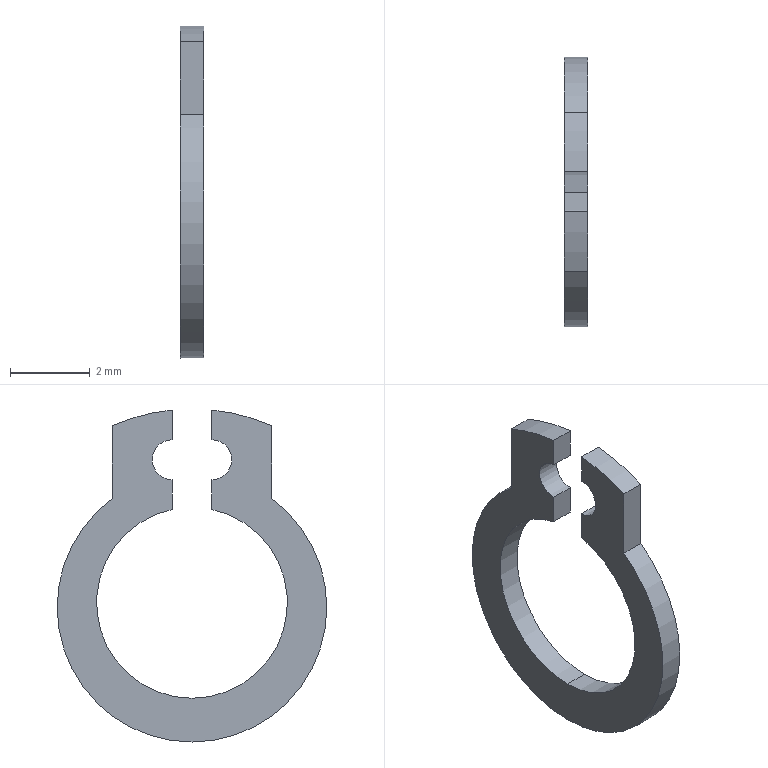Part | SolidWorks | features BaseBody 1 | 1 solid | 16 faces | box 0.6 x 6.78 x 8.347 mm | volume 12.837 mm3 | cylinder 8 | plane 8 | commonest cylinder face diameters 1 x2 4.8 x2 6.78 x2 9.965 x2
STEP:
#1=CARTESIAN_POINT('',(487.737,38.215,67.713));
#2=VERTEX_POINT('',#1);
#3=CARTESIAN_POINT('',(487.737,37.715,62.966));
#4=VERTEX_POINT('',#3);
#5=CARTESIAN_POINT('',(487.737,37.715,65.366));
#6=DIRECTION('',(-1.,0.,-0.000000013));
#7=DIRECTION('',(0.000000013,0.,-1.));
#8=AXIS2_PLACEMENT_3D('',#5,#6,#7);
#9=CIRCLE('',#8,2.4);
#10=EDGE_CURVE('',#2,#4,#9,.T.);
#11=ORIENTED_EDGE('',*,*,#10,.T.);
#12=CARTESIAN_POINT('',(488.337,37.715,62.966));
#13=VERTEX_POINT('',#12);
#14=CARTESIAN_POINT('',(487.737,37.715,62.966));
#15=DIRECTION('',(1.,0.,0.000000013));
#16=VECTOR('',#15,1000.);
#17=LINE('',#14,#16);
#18=EDGE_CURVE('',#4,#13,#17,.T.);
#19=ORIENTED_EDGE('',*,*,#18,.T.);
#20=CARTESIAN_POINT('',(488.337,38.215,67.713));
#21=VERTEX_POINT('',#20);
#22=CARTESIAN_POINT('',(488.337,37.715,65.366));
#23=DIRECTION('',(1.,0.,0.000000013));
#24=DIRECTION('',(0.000000013,0.,-1.));
#25=AXIS2_PLACEMENT_3D('',#22,#23,#24);
#26=CIRCLE('',#25,2.4);
#27=EDGE_CURVE('',#13,#21,#26,.T.);
#28=ORIENTED_EDGE('',*,*,#27,.T.);
#29=CARTESIAN_POINT('',(488.037,38.215,67.713));
#30=DIRECTION('',(-1.,0.,-0.000000013));
#31=VECTOR('',#30,1000.);
#32=LINE('',#29,#31);
#33=EDGE_CURVE('',#21,#2,#32,.T.);
#34=ORIENTED_EDGE('',*,*,#33,.T.);
#35=EDGE_LOOP('',(#11,#19,#28,#34));
#36=FACE_OUTER_BOUND('',#35,.T.);
#37=CARTESIAN_POINT('',(487.737,37.715,65.366));
#38=DIRECTION('',(1.,0.,0.000000013));
#39=DIRECTION('',(0.000000013,0.,-1.));
#40=AXIS2_PLACEMENT_3D('',#37,#38,#39);
#41=CYLINDRICAL_SURFACE('',#40,2.4);
#42=ADVANCED_FACE('',(#36),#41,.F.);
#43=CARTESIAN_POINT('',(487.737,35.715,67.993));
#44=VERTEX_POINT('',#43);
#45=CARTESIAN_POINT('',(487.737,37.715,61.866));
#46=VERTEX_POINT('',#45);
#47=CARTESIAN_POINT('',(487.737,37.715,65.256));
#48=DIRECTION('',(1.,0.,0.000000013));
#49=DIRECTION('',(0.000000013,0.,-1.));
#50=AXIS2_PLACEMENT_3D('',#47,#48,#49);
#51=CIRCLE('',#50,3.39);
#52=EDGE_CURVE('',#44,#46,#51,.T.);
#53=ORIENTED_EDGE('',*,*,#52,.T.);
#54=CARTESIAN_POINT('',(488.337,37.715,61.866));
#55=VERTEX_POINT('',#54);
#56=CARTESIAN_POINT('',(487.737,37.715,61.866));
#57=DIRECTION('',(1.,0.,0.000000013));
#58=VECTOR('',#57,1000.);
#59=LINE('',#56,#58);
#60=EDGE_CURVE('',#46,#55,#59,.T.);
#61=ORIENTED_EDGE('',*,*,#60,.T.);
#62=CARTESIAN_POINT('',(488.337,35.715,67.993));
#63=VERTEX_POINT('',#62);
#64=CARTESIAN_POINT('',(488.337,37.715,65.256));
#65=DIRECTION('',(1.,0.,0.000000013));
#66=DIRECTION('',(0.000000013,0.,-1.));
#67=AXIS2_PLACEMENT_3D('',#64,#65,#66);
#68=CIRCLE('',#67,3.39);
#69=EDGE_CURVE('',#63,#55,#68,.T.);
#70=ORIENTED_EDGE('',*,*,#69,.F.);
#71=CARTESIAN_POINT('',(488.037,35.715,67.993));
#72=DIRECTION('',(1.,0.,0.000000013));
#73=VECTOR('',#72,1000.);
#74=LINE('',#71,#73);
#75=EDGE_CURVE('',#44,#63,#74,.T.);
#76=ORIENTED_EDGE('',*,*,#75,.F.);
#77=EDGE_LOOP('',(#53,#61,#70,#76));
#78=FACE_OUTER_BOUND('',#77,.T.);
#79=CARTESIAN_POINT('',(487.737,37.715,65.256));
#80=DIRECTION('',(1.,0.,0.000000013));
#81=DIRECTION('',(0.000000013,0.,-1.));
#82=AXIS2_PLACEMENT_3D('',#79,#80,#81);
#83=CYLINDRICAL_SURFACE('',#82,3.39);
#84=ADVANCED_FACE('',(#78),#83,.T.);
#85=CARTESIAN_POINT('',(487.737,37.215,68.463));
#86=VERTEX_POINT('',#85);
#87=CARTESIAN_POINT('',(487.737,37.215,69.463));
#88=VERTEX_POINT('',#87);
#89=CARTESIAN_POINT('',(487.737,37.215,68.963));
#90=DIRECTION('',(-1.,0.,-0.000000013));
#91=DIRECTION('',(0.000000013,0.,-1.));
#92=AXIS2_PLACEMENT_3D('',#89,#90,#91);
#93=CIRCLE('',#92,0.5);
#94=EDGE_CURVE('',#86,#88,#93,.T.);
#95=ORIENTED_EDGE('',*,*,#94,.F.);
#96=CARTESIAN_POINT('',(487.737,37.215,67.713));
#97=VERTEX_POINT('',#96);
#98=CARTESIAN_POINT('',(487.737,37.215,66.04));
#99=DIRECTION('',(-0.000000013,0.,1.));
#100=VECTOR('',#99,1000.);
#101=LINE('',#98,#100);
#102=EDGE_CURVE('',#97,#86,#101,.T.);
#103=ORIENTED_EDGE('',*,*,#102,.F.);
#104=CARTESIAN_POINT('',(487.737,37.715,65.366));
#105=DIRECTION('',(-1.,0.,-0.000000013));
#106=DIRECTION('',(0.000000013,0.,-1.));
#107=AXIS2_PLACEMENT_3D('',#104,#105,#106);
#108=CIRCLE('',#107,2.4);
#109=EDGE_CURVE('',#4,#97,#108,.T.);
#110=ORIENTED_EDGE('',*,*,#109,.F.);
#111=ORIENTED_EDGE('',*,*,#10,.F.);
#112=CARTESIAN_POINT('',(487.737,38.215,68.463));
#113=VERTEX_POINT('',#112);
#114=CARTESIAN_POINT('',(487.737,38.215,66.04));
#115=DIRECTION('',(0.000000013,0.,-1.));
#116=VECTOR('',#115,1000.);
#117=LINE('',#114,#116);
#118=EDGE_CURVE('',#113,#2,#117,.T.);
#119=ORIENTED_EDGE('',*,*,#118,.F.);
#120=CARTESIAN_POINT('',(487.737,38.215,69.463));
#121=VERTEX_POINT('',#120);
#122=CARTESIAN_POINT('',(487.737,38.215,68.963));
#123=DIRECTION('',(-1.,0.,-0.000000013));
#124=DIRECTION('',(0.000000013,0.,-1.));
#125=AXIS2_PLACEMENT_3D('',#122,#123,#124);
#126=CIRCLE('',#125,0.5);
#127=EDGE_CURVE('',#121,#113,#126,.T.);
#128=ORIENTED_EDGE('',*,*,#127,.F.);
#129=CARTESIAN_POINT('',(487.737,38.215,70.213));
#130=VERTEX_POINT('',#129);
#131=CARTESIAN_POINT('',(487.737,38.215,66.04));
#132=DIRECTION('',(0.000000013,0.,-1.));
#133=VECTOR('',#132,1000.);
#134=LINE('',#131,#133);
#135=EDGE_CURVE('',#130,#121,#134,.T.);
#136=ORIENTED_EDGE('',*,*,#135,.F.);
#137=CARTESIAN_POINT('',(487.737,39.715,69.819));
#138=VERTEX_POINT('',#137);
#139=CARTESIAN_POINT('',(487.737,37.715,65.256));
#140=DIRECTION('',(1.,0.,0.000000013));
#141=DIRECTION('',(0.000000013,0.,-1.));
#142=AXIS2_PLACEMENT_3D('',#139,#140,#141);
#143=CIRCLE('',#142,4.982);
#144=EDGE_CURVE('',#138,#130,#143,.T.);
#145=ORIENTED_EDGE('',*,*,#144,.F.);
#146=CARTESIAN_POINT('',(487.737,39.715,67.993));
#147=VERTEX_POINT('',#146);
#148=CARTESIAN_POINT('',(487.737,39.715,66.04));
#149=DIRECTION('',(-0.000000013,0.,1.));
#150=VECTOR('',#149,1000.);
#151=LINE('',#148,#150);
#152=EDGE_CURVE('',#147,#138,#151,.T.);
#153=ORIENTED_EDGE('',*,*,#152,.F.);
#154=CARTESIAN_POINT('',(487.737,37.715,65.256));
#155=DIRECTION('',(1.,0.,0.000000013));
#156=DIRECTION('',(0.000000013,0.,-1.));
#157=AXIS2_PLACEMENT_3D('',#154,#155,#156);
#158=CIRCLE('',#157,3.39);
#159=EDGE_CURVE('',#46,#147,#158,.T.);
#160=ORIENTED_EDGE('',*,*,#159,.F.);
#161=ORIENTED_EDGE('',*,*,#52,.F.);
#162=CARTESIAN_POINT('',(487.737,35.715,69.819));
#163=VERTEX_POINT('',#162);
#164=CARTESIAN_POINT('',(487.737,35.715,66.04));
#165=DIRECTION('',(0.000000013,0.,-1.));
#166=VECTOR('',#165,1000.);
#167=LINE('',#164,#166);
#168=EDGE_CURVE('',#163,#44,#167,.T.);
#169=ORIENTED_EDGE('',*,*,#168,.F.);
#170=CARTESIAN_POINT('',(487.737,37.215,70.213));
#171=VERTEX_POINT('',#170);
#172=CARTESIAN_POINT('',(487.737,37.715,65.256));
#173=DIRECTION('',(1.,0.,0.000000013));
#174=DIRECTION('',(0.000000013,0.,-1.));
#175=AXIS2_PLACEMENT_3D('',#172,#173,#174);
#176=CIRCLE('',#175,4.982);
#177=EDGE_CURVE('',#171,#163,#176,.T.);
#178=ORIENTED_EDGE('',*,*,#177,.F.);
#179=CARTESIAN_POINT('',(487.737,37.215,66.04));
#180=DIRECTION('',(-0.000000013,0.,1.));
#181=VECTOR('',#180,1000.);
#182=LINE('',#179,#181);
#183=EDGE_CURVE('',#88,#171,#182,.T.);
#184=ORIENTED_EDGE('',*,*,#183,.F.);
#185=EDGE_LOOP('',(#95,#103,#110,#111,#119,#128,#136,#145,#153,#160,#161,#169,#178,#184));
#186=FACE_OUTER_BOUND('',#185,.T.);
#187=CARTESIAN_POINT('',(487.737,41.317,70.38));
#188=DIRECTION('',(1.,0.,0.000000013));
#189=DIRECTION('',(0.,-1.,0.));
#190=AXIS2_PLACEMENT_3D('',#187,#188,#189);
#191=PLANE('',#190);
#192=ADVANCED_FACE('',(#186),#191,.F.);
#193=CARTESIAN_POINT('',(488.337,37.215,69.463));
#194=VERTEX_POINT('',#193);
#195=CARTESIAN_POINT('',(488.037,37.215,69.463));
#196=DIRECTION('',(1.,0.,0.000000013));
#197=VECTOR('',#196,1000.);
#198=LINE('',#195,#197);
#199=EDGE_CURVE('',#88,#194,#198,.T.);
#200=ORIENTED_EDGE('',*,*,#199,.T.);
#201=CARTESIAN_POINT('',(488.337,37.215,68.463));
#202=VERTEX_POINT('',#201);
#203=CARTESIAN_POINT('',(488.337,37.215,68.963));
#204=DIRECTION('',(-1.,0.,-0.000000013));
#205=DIRECTION('',(0.000000013,0.,-1.));
#206=AXIS2_PLACEMENT_3D('',#203,#204,#205);
#207=CIRCLE('',#206,0.5);
#208=EDGE_CURVE('',#202,#194,#207,.T.);
#209=ORIENTED_EDGE('',*,*,#208,.F.);
#210=CARTESIAN_POINT('',(488.037,37.215,68.463));
#211=DIRECTION('',(-1.,0.,-0.000000013));
#212=VECTOR('',#211,1000.);
#213=LINE('',#210,#212);
#214=EDGE_CURVE('',#202,#86,#213,.T.);
#215=ORIENTED_EDGE('',*,*,#214,.T.);
#216=ORIENTED_EDGE('',*,*,#94,.T.);
#217=EDGE_LOOP('',(#200,#209,#215,#216));
#218=FACE_OUTER_BOUND('',#217,.T.);
#219=CARTESIAN_POINT('',(487.737,37.215,68.963));
#220=DIRECTION('',(1.,0.,0.000000013));
#221=DIRECTION('',(0.000000013,0.,-1.));
#222=AXIS2_PLACEMENT_3D('',#219,#220,#221);
#223=CYLINDRICAL_SURFACE('',#222,0.5);
#224=ADVANCED_FACE('',(#218),#223,.F.);
#225=CARTESIAN_POINT('',(488.337,37.215,67.713));
#226=VERTEX_POINT('',#225);
#227=CARTESIAN_POINT('',(488.037,37.215,67.713));
#228=DIRECTION('',(-1.,0.,-0.000000013));
#229=VECTOR('',#228,1000.);
#230=LINE('',#227,#229);
#231=EDGE_CURVE('',#226,#97,#230,.T.);
#232=ORIENTED_EDGE('',*,*,#231,.T.);
#233=ORIENTED_EDGE('',*,*,#102,.T.);
#234=ORIENTED_EDGE('',*,*,#214,.F.);
#235=CARTESIAN_POINT('',(488.337,37.215,66.04));
#236=DIRECTION('',(-0.000000013,0.,1.));
#237=VECTOR('',#236,1000.);
#238=LINE('',#235,#237);
#239=EDGE_CURVE('',#226,#202,#238,.T.);
#240=ORIENTED_EDGE('',*,*,#239,.F.);
#241=EDGE_LOOP('',(#232,#233,#234,#240));
#242=FACE_OUTER_BOUND('',#241,.T.);
#243=CARTESIAN_POINT('',(487.724,37.215,67.663));
#244=DIRECTION('',(0.,1.,0.));
#245=DIRECTION('',(-0.000000013,0.,1.));
#246=AXIS2_PLACEMENT_3D('',#243,#244,#245);
#247=PLANE('',#246);
#248=ADVANCED_FACE('',(#242),#247,.T.);
#249=ORIENTED_EDGE('',*,*,#18,.F.);
#250=ORIENTED_EDGE('',*,*,#109,.T.);
#251=ORIENTED_EDGE('',*,*,#231,.F.);
#252=CARTESIAN_POINT('',(488.337,37.715,65.366));
#253=DIRECTION('',(1.,0.,0.000000013));
#254=DIRECTION('',(0.000000013,0.,-1.));
#255=AXIS2_PLACEMENT_3D('',#252,#253,#254);
#256=CIRCLE('',#255,2.4);
#257=EDGE_CURVE('',#226,#13,#256,.T.);
#258=ORIENTED_EDGE('',*,*,#257,.T.);
#259=EDGE_LOOP('',(#249,#250,#251,#258));
#260=FACE_OUTER_BOUND('',#259,.T.);
#261=CARTESIAN_POINT('',(487.737,37.715,65.366));
#262=DIRECTION('',(1.,0.,0.000000013));
#263=DIRECTION('',(0.000000013,0.,-1.));
#264=AXIS2_PLACEMENT_3D('',#261,#262,#263);
#265=CYLINDRICAL_SURFACE('',#264,2.4);
#266=ADVANCED_FACE('',(#260),#265,.F.);
#267=ORIENTED_EDGE('',*,*,#33,.F.);
#268=CARTESIAN_POINT('',(488.337,38.215,68.463));
#269=VERTEX_POINT('',#268);
#270=CARTESIAN_POINT('',(488.337,38.215,68.963));
#271=DIRECTION('',(-0.000000013,0.,1.));
#272=VECTOR('',#271,1000.);
#273=LINE('',#270,#272);
#274=EDGE_CURVE('',#21,#269,#273,.T.);
#275=ORIENTED_EDGE('',*,*,#274,.T.);
#276=CARTESIAN_POINT('',(488.037,38.215,68.463));
#277=DIRECTION('',(-1.,0.,-0.000000013));
#278=VECTOR('',#277,1000.);
#279=LINE('',#276,#278);
#280=EDGE_CURVE('',#269,#113,#279,.T.);
#281=ORIENTED_EDGE('',*,*,#280,.T.);
#282=ORIENTED_EDGE('',*,*,#118,.T.);
#283=EDGE_LOOP('',(#267,#275,#281,#282));
#284=FACE_OUTER_BOUND('',#283,.T.);
#285=CARTESIAN_POINT('',(487.724,38.215,70.263));
#286=DIRECTION('',(0.,-1.,0.));
#287=DIRECTION('',(0.000000013,0.,-1.));
#288=AXIS2_PLACEMENT_3D('',#285,#286,#287);
#289=PLANE('',#288);
#290=ADVANCED_FACE('',(#284),#289,.T.);
#291=ORIENTED_EDGE('',*,*,#280,.F.);
#292=CARTESIAN_POINT('',(488.337,38.215,69.463));
#293=VERTEX_POINT('',#292);
#294=CARTESIAN_POINT('',(488.337,38.215,68.963));
#295=DIRECTION('',(1.,0.,0.000000013));
#296=DIRECTION('',(0.000000013,0.,-1.));
#297=AXIS2_PLACEMENT_3D('',#294,#295,#296);
#298=CIRCLE('',#297,0.5);
#299=EDGE_CURVE('',#269,#293,#298,.T.);
#300=ORIENTED_EDGE('',*,*,#299,.T.);
#301=CARTESIAN_POINT('',(488.037,38.215,69.463));
#302=DIRECTION('',(-1.,0.,-0.000000013));
#303=VECTOR('',#302,1000.);
#304=LINE('',#301,#303);
#305=EDGE_CURVE('',#293,#121,#304,.T.);
#306=ORIENTED_EDGE('',*,*,#305,.T.);
#307=ORIENTED_EDGE('',*,*,#127,.T.);
#308=EDGE_LOOP('',(#291,#300,#306,#307));
#309=FACE_OUTER_BOUND('',#308,.T.);
#310=CARTESIAN_POINT('',(487.737,38.215,68.963));
#311=DIRECTION('',(1.,0.,0.000000013));
#312=DIRECTION('',(0.000000013,0.,-1.));
#313=AXIS2_PLACEMENT_3D('',#310,#311,#312);
#314=CYLINDRICAL_SURFACE('',#313,0.5);
#315=ADVANCED_FACE('',(#309),#314,.F.);
#316=CARTESIAN_POINT('',(488.337,38.215,70.213));
#317=VERTEX_POINT('',#316);
#318=CARTESIAN_POINT('',(488.037,38.215,70.213));
#319=DIRECTION('',(-1.,0.,-0.000000013));
#320=VECTOR('',#319,1000.);
#321=LINE('',#318,#320);
#322=EDGE_CURVE('',#317,#130,#321,.T.);
#323=ORIENTED_EDGE('',*,*,#322,.T.);
#324=ORIENTED_EDGE('',*,*,#135,.T.);
#325=ORIENTED_EDGE('',*,*,#305,.F.);
#326=CARTESIAN_POINT('',(488.337,38.215,68.963));
#327=DIRECTION('',(-0.000000013,0.,1.));
#328=VECTOR('',#327,1000.);
#329=LINE('',#326,#328);
#330=EDGE_CURVE('',#293,#317,#329,.T.);
#331=ORIENTED_EDGE('',*,*,#330,.T.);
#332=EDGE_LOOP('',(#323,#324,#325,#331));
#333=FACE_OUTER_BOUND('',#332,.T.);
#334=CARTESIAN_POINT('',(487.724,38.215,70.263));
#335=DIRECTION('',(0.,-1.,0.));
#336=DIRECTION('',(0.000000013,0.,-1.));
#337=AXIS2_PLACEMENT_3D('',#334,#335,#336);
#338=PLANE('',#337);
#339=ADVANCED_FACE('',(#333),#338,.T.);
#340=ORIENTED_EDGE('',*,*,#322,.F.);
#341=CARTESIAN_POINT('',(488.337,39.715,69.819));
#342=VERTEX_POINT('',#341);
#343=CARTESIAN_POINT('',(488.337,37.715,65.256));
#344=DIRECTION('',(1.,0.,0.000000013));
#345=DIRECTION('',(0.000000013,0.,-1.));
#346=AXIS2_PLACEMENT_3D('',#343,#344,#345);
#347=CIRCLE('',#346,4.982);
#348=EDGE_CURVE('',#342,#317,#347,.T.);
#349=ORIENTED_EDGE('',*,*,#348,.F.);
#350=CARTESIAN_POINT('',(488.037,39.715,69.819));
#351=DIRECTION('',(1.,0.,0.000000013));
#352=VECTOR('',#351,1000.);
#353=LINE('',#350,#352);
#354=EDGE_CURVE('',#138,#342,#353,.T.);
#355=ORIENTED_EDGE('',*,*,#354,.F.);
#356=ORIENTED_EDGE('',*,*,#144,.T.);
#357=EDGE_LOOP('',(#340,#349,#355,#356));
#358=FACE_OUTER_BOUND('',#357,.T.);
#359=CARTESIAN_POINT('',(487.737,37.715,65.256));
#360=DIRECTION('',(1.,0.,0.000000013));
#361=DIRECTION('',(0.000000013,0.,-1.));
#362=AXIS2_PLACEMENT_3D('',#359,#360,#361);
#363=CYLINDRICAL_SURFACE('',#362,4.982);
#364=ADVANCED_FACE('',(#358),#363,.T.);
#365=CARTESIAN_POINT('',(488.337,39.715,67.993));
#366=VERTEX_POINT('',#365);
#367=CARTESIAN_POINT('',(488.337,39.715,68.906));
#368=DIRECTION('',(0.000000013,0.,-1.));
#369=VECTOR('',#368,1000.);
#370=LINE('',#367,#369);
#371=EDGE_CURVE('',#342,#366,#370,.T.);
#372=ORIENTED_EDGE('',*,*,#371,.T.);
#373=CARTESIAN_POINT('',(488.037,39.715,67.993));
#374=DIRECTION('',(-1.,0.,-0.000000013));
#375=VECTOR('',#374,1000.);
#376=LINE('',#373,#375);
#377=EDGE_CURVE('',#366,#147,#376,.T.);
#378=ORIENTED_EDGE('',*,*,#377,.T.);
#379=ORIENTED_EDGE('',*,*,#152,.T.);
#380=ORIENTED_EDGE('',*,*,#354,.T.);
#381=EDGE_LOOP('',(#372,#378,#379,#380));
#382=FACE_OUTER_BOUND('',#381,.T.);
#383=CARTESIAN_POINT('',(487.724,39.715,67.957));
#384=DIRECTION('',(0.,1.,0.));
#385=DIRECTION('',(-0.000000013,0.,1.));
#386=AXIS2_PLACEMENT_3D('',#383,#384,#385);
#387=PLANE('',#386);
#388=ADVANCED_FACE('',(#382),#387,.T.);
#389=ORIENTED_EDGE('',*,*,#60,.F.);
#390=ORIENTED_EDGE('',*,*,#159,.T.);
#391=ORIENTED_EDGE('',*,*,#377,.F.);
#392=CARTESIAN_POINT('',(488.337,37.715,65.256));
#393=DIRECTION('',(1.,0.,0.000000013));
#394=DIRECTION('',(0.000000013,0.,-1.));
#395=AXIS2_PLACEMENT_3D('',#392,#393,#394);
#396=CIRCLE('',#395,3.39);
#397=EDGE_CURVE('',#55,#366,#396,.T.);
#398=ORIENTED_EDGE('',*,*,#397,.F.);
#399=EDGE_LOOP('',(#389,#390,#391,#398));
#400=FACE_OUTER_BOUND('',#399,.T.);
#401=CARTESIAN_POINT('',(487.737,37.715,65.256));
#402=DIRECTION('',(1.,0.,0.000000013));
#403=DIRECTION('',(0.000000013,0.,-1.));
#404=AXIS2_PLACEMENT_3D('',#401,#402,#403);
#405=CYLINDRICAL_SURFACE('',#404,3.39);
#406=ADVANCED_FACE('',(#400),#405,.T.);
#407=CARTESIAN_POINT('',(488.337,35.715,69.819));
#408=VERTEX_POINT('',#407);
#409=CARTESIAN_POINT('',(488.337,35.715,68.906));
#410=DIRECTION('',(-0.000000013,0.,1.));
#411=VECTOR('',#410,1000.);
#412=LINE('',#409,#411);
#413=EDGE_CURVE('',#63,#408,#412,.T.);
#414=ORIENTED_EDGE('',*,*,#413,.T.);
#415=CARTESIAN_POINT('',(488.037,35.715,69.819));
#416=DIRECTION('',(-1.,0.,-0.000000013));
#417=VECTOR('',#416,1000.);
#418=LINE('',#415,#417);
#419=EDGE_CURVE('',#408,#163,#418,.T.);
#420=ORIENTED_EDGE('',*,*,#419,.T.);
#421=ORIENTED_EDGE('',*,*,#168,.T.);
#422=ORIENTED_EDGE('',*,*,#75,.T.);
#423=EDGE_LOOP('',(#414,#420,#421,#422));
#424=FACE_OUTER_BOUND('',#423,.T.);
#425=CARTESIAN_POINT('',(487.724,35.715,69.856));
#426=DIRECTION('',(0.,-1.,0.));
#427=DIRECTION('',(0.000000013,0.,-1.));
#428=AXIS2_PLACEMENT_3D('',#425,#426,#427);
#429=PLANE('',#428);
#430=ADVANCED_FACE('',(#424),#429,.T.);
#431=ORIENTED_EDGE('',*,*,#419,.F.);
#432=CARTESIAN_POINT('',(488.337,37.215,70.213));
#433=VERTEX_POINT('',#432);
#434=CARTESIAN_POINT('',(488.337,37.715,65.256));
#435=DIRECTION('',(1.,0.,0.000000013));
#436=DIRECTION('',(0.000000013,0.,-1.));
#437=AXIS2_PLACEMENT_3D('',#434,#435,#436);
#438=CIRCLE('',#437,4.982);
#439=EDGE_CURVE('',#433,#408,#438,.T.);
#440=ORIENTED_EDGE('',*,*,#439,.F.);
#441=CARTESIAN_POINT('',(488.037,37.215,70.213));
#442=DIRECTION('',(1.,0.,0.000000013));
#443=VECTOR('',#442,1000.);
#444=LINE('',#441,#443);
#445=EDGE_CURVE('',#171,#433,#444,.T.);
#446=ORIENTED_EDGE('',*,*,#445,.F.);
#447=ORIENTED_EDGE('',*,*,#177,.T.);
#448=EDGE_LOOP('',(#431,#440,#446,#447));
#449=FACE_OUTER_BOUND('',#448,.T.);
#450=CARTESIAN_POINT('',(487.737,37.715,65.256));
#451=DIRECTION('',(1.,0.,0.000000013));
#452=DIRECTION('',(0.000000013,0.,-1.));
#453=AXIS2_PLACEMENT_3D('',#450,#451,#452);
#454=CYLINDRICAL_SURFACE('',#453,4.982);
#455=ADVANCED_FACE('',(#449),#454,.T.);
#456=ORIENTED_EDGE('',*,*,#445,.T.);
#457=CARTESIAN_POINT('',(488.337,37.215,68.963));
#458=DIRECTION('',(0.000000013,0.,-1.));
#459=VECTOR('',#458,1000.);
#460=LINE('',#457,#459);
#461=EDGE_CURVE('',#433,#194,#460,.T.);
#462=ORIENTED_EDGE('',*,*,#461,.T.);
#463=ORIENTED_EDGE('',*,*,#199,.F.);
#464=ORIENTED_EDGE('',*,*,#183,.T.);
#465=EDGE_LOOP('',(#456,#462,#463,#464));
#466=FACE_OUTER_BOUND('',#465,.T.);
#467=CARTESIAN_POINT('',(487.724,37.215,67.663));
#468=DIRECTION('',(0.,1.,0.));
#469=DIRECTION('',(-0.000000013,0.,1.));
#470=AXIS2_PLACEMENT_3D('',#467,#468,#469);
#471=PLANE('',#470);
#472=ADVANCED_FACE('',(#466),#471,.T.);
#473=ORIENTED_EDGE('',*,*,#257,.F.);
#474=ORIENTED_EDGE('',*,*,#239,.T.);
#475=ORIENTED_EDGE('',*,*,#208,.T.);
#476=ORIENTED_EDGE('',*,*,#461,.F.);
#477=ORIENTED_EDGE('',*,*,#439,.T.);
#478=ORIENTED_EDGE('',*,*,#413,.F.);
#479=ORIENTED_EDGE('',*,*,#69,.T.);
#480=ORIENTED_EDGE('',*,*,#397,.T.);
#481=ORIENTED_EDGE('',*,*,#371,.F.);
#482=ORIENTED_EDGE('',*,*,#348,.T.);
#483=ORIENTED_EDGE('',*,*,#330,.F.);
#484=ORIENTED_EDGE('',*,*,#299,.F.);
#485=ORIENTED_EDGE('',*,*,#274,.F.);
#486=ORIENTED_EDGE('',*,*,#27,.F.);
#487=EDGE_LOOP('',(#473,#474,#475,#476,#477,#478,#479,#480,#481,#482,#483,#484,#485,#486));
#488=FACE_OUTER_BOUND('',#487,.T.);
#489=CARTESIAN_POINT('',(488.337,41.32,70.38));
#490=DIRECTION('',(1.,0.,0.000000013));
#491=DIRECTION('',(0.,-1.,0.));
#492=AXIS2_PLACEMENT_3D('',#489,#490,#491);
#493=PLANE('',#492);
#494=ADVANCED_FACE('',(#488),#493,.T.);
#495=CLOSED_SHELL('',(#42,#84,#192,#224,#248,#266,#290,#315,#339,#364,#388,#406,#430,#455,#472,#494));
#496=MANIFOLD_SOLID_BREP('',#495);
#497=CARTESIAN_POINT('',(0.,0.,0.));
#498=DIRECTION('',(0.,0.,1.));
#499=DIRECTION('',(1.,0.,0.));
#500=AXIS2_PLACEMENT_3D('',#497,#498,#499);
#501=(LENGTH_UNIT()NAMED_UNIT(*)SI_UNIT(.MILLI.,.METRE.));
#502=UNCERTAINTY_MEASURE_WITH_UNIT(LENGTH_MEASURE(0.00001),#501,'','');
#503=(NAMED_UNIT(*)PLANE_ANGLE_UNIT()SI_UNIT($,.RADIAN.));
#504=(NAMED_UNIT(*)SI_UNIT($,.STERADIAN.)SOLID_ANGLE_UNIT());
#505=(GEOMETRIC_REPRESENTATION_CONTEXT(3)GLOBAL_UNCERTAINTY_ASSIGNED_CONTEXT((#502))GLOBAL_UNIT_ASSIGNED_CONTEXT((#501,#503,#504))REPRESENTATION_CONTEXT('',''));
#506=ADVANCED_BREP_SHAPE_REPRESENTATION('',(#496,#500),#505);